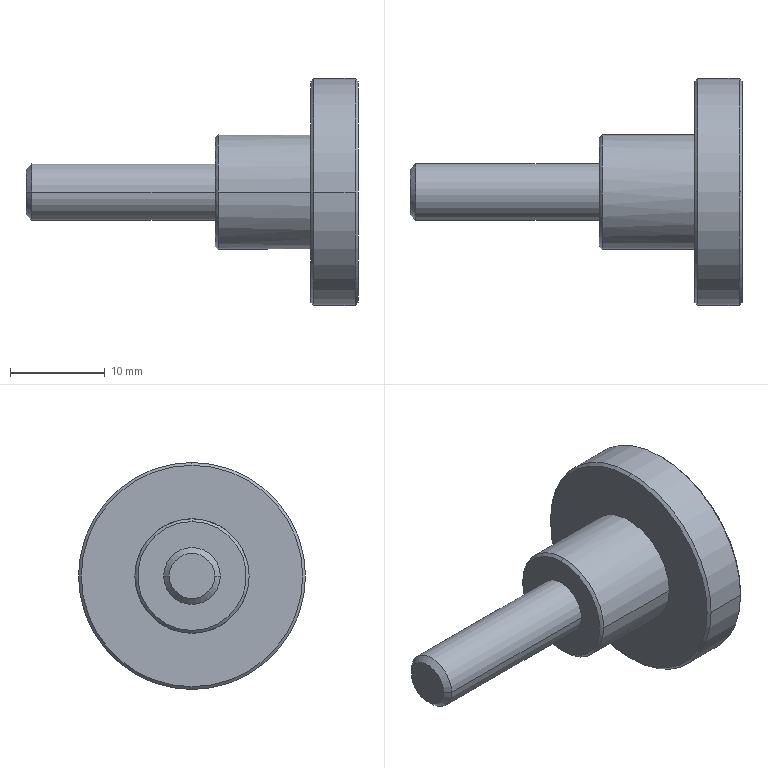Part | SolidWorks | features BaseBody 1 | 1 solid | 18 faces | box 35.1 x 24 x 24 mm | volume 3977 mm3 | cone 8 | cylinder 6 | plane 4 | commonest cylinder face diameters 6 x2 12.1 x2 24 x2
STEP:
#1=CARTESIAN_POINT('',(35.1,0.,-11.7));
#2=VERTEX_POINT('',#1);
#3=CARTESIAN_POINT('',(35.1,0.,11.7));
#4=VERTEX_POINT('',#3);
#5=CARTESIAN_POINT('',(35.1,0.,0.));
#6=DIRECTION('',(1.,0.,0.));
#7=DIRECTION('',(0.,0.,1.));
#8=AXIS2_PLACEMENT_3D('',#5,#6,#7);
#9=CIRCLE('',#8,11.7);
#10=EDGE_CURVE('',#2,#4,#9,.T.);
#11=ORIENTED_EDGE('',*,*,#10,.F.);
#12=CARTESIAN_POINT('',(34.8,0.,-12.));
#13=VERTEX_POINT('',#12);
#14=CARTESIAN_POINT('',(34.8,0.,-12.));
#15=DIRECTION('',(-0.7071,0.,-0.7071));
#16=VECTOR('',#15,1000.);
#17=LINE('',#14,#16);
#18=EDGE_CURVE('',#2,#13,#17,.T.);
#19=ORIENTED_EDGE('',*,*,#18,.T.);
#20=CARTESIAN_POINT('',(34.8,12.,0.));
#21=VERTEX_POINT('',#20);
#22=CARTESIAN_POINT('',(34.8,0.,0.));
#23=DIRECTION('',(1.,0.,0.));
#24=DIRECTION('',(0.,-1.,0.));
#25=AXIS2_PLACEMENT_3D('',#22,#23,#24);
#26=CIRCLE('',#25,12.);
#27=EDGE_CURVE('',#13,#21,#26,.T.);
#28=ORIENTED_EDGE('',*,*,#27,.T.);
#29=CARTESIAN_POINT('',(34.8,0.,12.));
#30=VERTEX_POINT('',#29);
#31=CARTESIAN_POINT('',(34.8,0.,0.));
#32=DIRECTION('',(1.,0.,0.));
#33=DIRECTION('',(0.,-1.,0.));
#34=AXIS2_PLACEMENT_3D('',#31,#32,#33);
#35=CIRCLE('',#34,12.);
#36=EDGE_CURVE('',#21,#30,#35,.T.);
#37=ORIENTED_EDGE('',*,*,#36,.T.);
#38=CARTESIAN_POINT('',(34.8,0.,12.));
#39=DIRECTION('',(-0.7071,0.,0.7071));
#40=VECTOR('',#39,1000.);
#41=LINE('',#38,#40);
#42=EDGE_CURVE('',#4,#30,#41,.T.);
#43=ORIENTED_EDGE('',*,*,#42,.F.);
#44=EDGE_LOOP('',(#11,#19,#28,#37,#43));
#45=FACE_OUTER_BOUND('',#44,.T.);
#46=CARTESIAN_POINT('',(34.8,0.,0.));
#47=DIRECTION('',(-1.,0.,0.));
#48=DIRECTION('',(0.,0.,1.));
#49=AXIS2_PLACEMENT_3D('',#46,#47,#48);
#50=CONICAL_SURFACE('',#49,12.,0.7854);
#51=ADVANCED_FACE('',(#45),#50,.T.);
#52=CARTESIAN_POINT('',(30.4,0.,12.));
#53=VERTEX_POINT('',#52);
#54=CARTESIAN_POINT('',(30.4,-12.,0.));
#55=VERTEX_POINT('',#54);
#56=CARTESIAN_POINT('',(30.4,0.,0.));
#57=DIRECTION('',(1.,0.,0.));
#58=DIRECTION('',(0.,1.,0.));
#59=AXIS2_PLACEMENT_3D('',#56,#57,#58);
#60=CIRCLE('',#59,12.);
#61=EDGE_CURVE('',#53,#55,#60,.T.);
#62=ORIENTED_EDGE('',*,*,#61,.T.);
#63=CARTESIAN_POINT('',(34.8,-12.,0.));
#64=VERTEX_POINT('',#63);
#65=CARTESIAN_POINT('',(35.1,-12.,0.));
#66=DIRECTION('',(1.,0.,0.));
#67=VECTOR('',#66,1000.);
#68=LINE('',#65,#67);
#69=EDGE_CURVE('',#55,#64,#68,.T.);
#70=ORIENTED_EDGE('',*,*,#69,.T.);
#71=CARTESIAN_POINT('',(34.8,0.,0.));
#72=DIRECTION('',(1.,0.,0.));
#73=DIRECTION('',(0.,-1.,0.));
#74=AXIS2_PLACEMENT_3D('',#71,#72,#73);
#75=CIRCLE('',#74,12.);
#76=EDGE_CURVE('',#30,#64,#75,.T.);
#77=ORIENTED_EDGE('',*,*,#76,.F.);
#78=ORIENTED_EDGE('',*,*,#36,.F.);
#79=CARTESIAN_POINT('',(30.4,12.,0.));
#80=VERTEX_POINT('',#79);
#81=CARTESIAN_POINT('',(35.1,12.,0.));
#82=DIRECTION('',(1.,0.,0.));
#83=VECTOR('',#82,1000.);
#84=LINE('',#81,#83);
#85=EDGE_CURVE('',#80,#21,#84,.T.);
#86=ORIENTED_EDGE('',*,*,#85,.F.);
#87=CARTESIAN_POINT('',(30.4,0.,0.));
#88=DIRECTION('',(1.,0.,0.));
#89=DIRECTION('',(0.,1.,0.));
#90=AXIS2_PLACEMENT_3D('',#87,#88,#89);
#91=CIRCLE('',#90,12.);
#92=EDGE_CURVE('',#80,#53,#91,.T.);
#93=ORIENTED_EDGE('',*,*,#92,.T.);
#94=EDGE_LOOP('',(#62,#70,#77,#78,#86,#93));
#95=FACE_OUTER_BOUND('',#94,.T.);
#96=CARTESIAN_POINT('',(35.1,0.,0.));
#97=DIRECTION('',(1.,0.,0.));
#98=DIRECTION('',(0.,1.,0.));
#99=AXIS2_PLACEMENT_3D('',#96,#97,#98);
#100=CYLINDRICAL_SURFACE('',#99,12.);
#101=ADVANCED_FACE('',(#95),#100,.T.);
#102=CARTESIAN_POINT('',(30.1,0.,-11.7));
#103=VERTEX_POINT('',#102);
#104=CARTESIAN_POINT('',(30.1,0.,11.7));
#105=VERTEX_POINT('',#104);
#106=CARTESIAN_POINT('',(30.1,0.,0.));
#107=DIRECTION('',(1.,0.,0.));
#108=DIRECTION('',(0.,0.,-1.));
#109=AXIS2_PLACEMENT_3D('',#106,#107,#108);
#110=CIRCLE('',#109,11.7);
#111=EDGE_CURVE('',#103,#105,#110,.T.);
#112=ORIENTED_EDGE('',*,*,#111,.T.);
#113=CARTESIAN_POINT('',(30.4,0.,12.));
#114=DIRECTION('',(0.7071,0.,0.7071));
#115=VECTOR('',#114,1000.);
#116=LINE('',#113,#115);
#117=EDGE_CURVE('',#105,#53,#116,.T.);
#118=ORIENTED_EDGE('',*,*,#117,.T.);
#119=ORIENTED_EDGE('',*,*,#92,.F.);
#120=CARTESIAN_POINT('',(30.4,0.,-12.));
#121=VERTEX_POINT('',#120);
#122=CARTESIAN_POINT('',(30.4,0.,0.));
#123=DIRECTION('',(1.,0.,0.));
#124=DIRECTION('',(0.,1.,0.));
#125=AXIS2_PLACEMENT_3D('',#122,#123,#124);
#126=CIRCLE('',#125,12.);
#127=EDGE_CURVE('',#121,#80,#126,.T.);
#128=ORIENTED_EDGE('',*,*,#127,.F.);
#129=CARTESIAN_POINT('',(30.4,0.,-12.));
#130=DIRECTION('',(0.7071,0.,-0.7071));
#131=VECTOR('',#130,1000.);
#132=LINE('',#129,#131);
#133=EDGE_CURVE('',#103,#121,#132,.T.);
#134=ORIENTED_EDGE('',*,*,#133,.F.);
#135=EDGE_LOOP('',(#112,#118,#119,#128,#134));
#136=FACE_OUTER_BOUND('',#135,.T.);
#137=CARTESIAN_POINT('',(30.4,0.,0.));
#138=DIRECTION('',(1.,0.,0.));
#139=DIRECTION('',(0.,0.,-1.));
#140=AXIS2_PLACEMENT_3D('',#137,#138,#139);
#141=CONICAL_SURFACE('',#140,12.,0.7854);
#142=ADVANCED_FACE('',(#136),#141,.T.);
#143=CARTESIAN_POINT('',(20.3,0.,6.05));
#144=VERTEX_POINT('',#143);
#145=CARTESIAN_POINT('',(20.3,-6.05,0.));
#146=VERTEX_POINT('',#145);
#147=CARTESIAN_POINT('',(20.3,0.,0.));
#148=DIRECTION('',(1.,0.,0.));
#149=DIRECTION('',(0.,1.,0.));
#150=AXIS2_PLACEMENT_3D('',#147,#148,#149);
#151=CIRCLE('',#150,6.05);
#152=EDGE_CURVE('',#144,#146,#151,.T.);
#153=ORIENTED_EDGE('',*,*,#152,.T.);
#154=CARTESIAN_POINT('',(30.1,-6.05,0.));
#155=VERTEX_POINT('',#154);
#156=CARTESIAN_POINT('',(35.1,-6.05,0.));
#157=DIRECTION('',(1.,0.,0.));
#158=VECTOR('',#157,1000.);
#159=LINE('',#156,#158);
#160=EDGE_CURVE('',#146,#155,#159,.T.);
#161=ORIENTED_EDGE('',*,*,#160,.T.);
#162=CARTESIAN_POINT('',(30.1,6.05,0.));
#163=VERTEX_POINT('',#162);
#164=CARTESIAN_POINT('',(30.1,0.,0.));
#165=DIRECTION('',(1.,0.,0.));
#166=DIRECTION('',(0.,1.,0.));
#167=AXIS2_PLACEMENT_3D('',#164,#165,#166);
#168=CIRCLE('',#167,6.05);
#169=EDGE_CURVE('',#163,#155,#168,.T.);
#170=ORIENTED_EDGE('',*,*,#169,.F.);
#171=CARTESIAN_POINT('',(20.3,6.05,0.));
#172=VERTEX_POINT('',#171);
#173=CARTESIAN_POINT('',(35.1,6.05,0.));
#174=DIRECTION('',(1.,0.,0.));
#175=VECTOR('',#174,1000.);
#176=LINE('',#173,#175);
#177=EDGE_CURVE('',#172,#163,#176,.T.);
#178=ORIENTED_EDGE('',*,*,#177,.F.);
#179=CARTESIAN_POINT('',(20.3,0.,0.));
#180=DIRECTION('',(1.,0.,0.));
#181=DIRECTION('',(0.,1.,0.));
#182=AXIS2_PLACEMENT_3D('',#179,#180,#181);
#183=CIRCLE('',#182,6.05);
#184=EDGE_CURVE('',#172,#144,#183,.T.);
#185=ORIENTED_EDGE('',*,*,#184,.T.);
#186=EDGE_LOOP('',(#153,#161,#170,#178,#185));
#187=FACE_OUTER_BOUND('',#186,.T.);
#188=CARTESIAN_POINT('',(35.1,0.,0.));
#189=DIRECTION('',(1.,0.,0.));
#190=DIRECTION('',(0.,1.,0.));
#191=AXIS2_PLACEMENT_3D('',#188,#189,#190);
#192=CYLINDRICAL_SURFACE('',#191,6.05);
#193=ADVANCED_FACE('',(#187),#192,.T.);
#194=CARTESIAN_POINT('',(20.,0.,-5.75));
#195=VERTEX_POINT('',#194);
#196=CARTESIAN_POINT('',(20.,0.,5.75));
#197=VERTEX_POINT('',#196);
#198=CARTESIAN_POINT('',(20.,0.,0.));
#199=DIRECTION('',(1.,0.,0.));
#200=DIRECTION('',(0.,0.,-1.));
#201=AXIS2_PLACEMENT_3D('',#198,#199,#200);
#202=CIRCLE('',#201,5.75);
#203=EDGE_CURVE('',#195,#197,#202,.T.);
#204=ORIENTED_EDGE('',*,*,#203,.T.);
#205=CARTESIAN_POINT('',(20.3,0.,6.05));
#206=DIRECTION('',(0.7071,0.,0.7071));
#207=VECTOR('',#206,1000.);
#208=LINE('',#205,#207);
#209=EDGE_CURVE('',#197,#144,#208,.T.);
#210=ORIENTED_EDGE('',*,*,#209,.T.);
#211=ORIENTED_EDGE('',*,*,#184,.F.);
#212=CARTESIAN_POINT('',(20.3,0.,-6.05));
#213=VERTEX_POINT('',#212);
#214=CARTESIAN_POINT('',(20.3,0.,0.));
#215=DIRECTION('',(1.,0.,0.));
#216=DIRECTION('',(0.,1.,0.));
#217=AXIS2_PLACEMENT_3D('',#214,#215,#216);
#218=CIRCLE('',#217,6.05);
#219=EDGE_CURVE('',#213,#172,#218,.T.);
#220=ORIENTED_EDGE('',*,*,#219,.F.);
#221=CARTESIAN_POINT('',(20.3,0.,-6.05));
#222=DIRECTION('',(0.7071,0.,-0.7071));
#223=VECTOR('',#222,1000.);
#224=LINE('',#221,#223);
#225=EDGE_CURVE('',#195,#213,#224,.T.);
#226=ORIENTED_EDGE('',*,*,#225,.F.);
#227=EDGE_LOOP('',(#204,#210,#211,#220,#226));
#228=FACE_OUTER_BOUND('',#227,.T.);
#229=CARTESIAN_POINT('',(20.3,0.,0.));
#230=DIRECTION('',(1.,0.,0.));
#231=DIRECTION('',(0.,0.,-1.));
#232=AXIS2_PLACEMENT_3D('',#229,#230,#231);
#233=CONICAL_SURFACE('',#232,6.05,0.7854);
#234=ADVANCED_FACE('',(#228),#233,.T.);
#235=CARTESIAN_POINT('',(0.6,3.,0.));
#236=VERTEX_POINT('',#235);
#237=CARTESIAN_POINT('',(0.6,-3.,0.));
#238=VERTEX_POINT('',#237);
#239=CARTESIAN_POINT('',(0.6,0.,0.));
#240=DIRECTION('',(1.,0.,0.));
#241=DIRECTION('',(0.,1.,0.));
#242=AXIS2_PLACEMENT_3D('',#239,#240,#241);
#243=CIRCLE('',#242,3.);
#244=EDGE_CURVE('',#236,#238,#243,.T.);
#245=ORIENTED_EDGE('',*,*,#244,.T.);
#246=CARTESIAN_POINT('',(20.,-3.,0.));
#247=VERTEX_POINT('',#246);
#248=CARTESIAN_POINT('',(35.1,-3.,0.));
#249=DIRECTION('',(1.,0.,0.));
#250=VECTOR('',#249,1000.);
#251=LINE('',#248,#250);
#252=EDGE_CURVE('',#238,#247,#251,.T.);
#253=ORIENTED_EDGE('',*,*,#252,.T.);
#254=CARTESIAN_POINT('',(20.,3.,0.));
#255=VERTEX_POINT('',#254);
#256=CARTESIAN_POINT('',(20.,0.,0.));
#257=DIRECTION('',(1.,0.,0.));
#258=DIRECTION('',(0.,1.,0.));
#259=AXIS2_PLACEMENT_3D('',#256,#257,#258);
#260=CIRCLE('',#259,3.);
#261=EDGE_CURVE('',#255,#247,#260,.T.);
#262=ORIENTED_EDGE('',*,*,#261,.F.);
#263=CARTESIAN_POINT('',(35.1,3.,0.));
#264=DIRECTION('',(1.,0.,0.));
#265=VECTOR('',#264,1000.);
#266=LINE('',#263,#265);
#267=EDGE_CURVE('',#236,#255,#266,.T.);
#268=ORIENTED_EDGE('',*,*,#267,.F.);
#269=EDGE_LOOP('',(#245,#253,#262,#268));
#270=FACE_OUTER_BOUND('',#269,.T.);
#271=CARTESIAN_POINT('',(35.1,0.,0.));
#272=DIRECTION('',(1.,0.,0.));
#273=DIRECTION('',(0.,1.,0.));
#274=AXIS2_PLACEMENT_3D('',#271,#272,#273);
#275=CYLINDRICAL_SURFACE('',#274,3.);
#276=ADVANCED_FACE('',(#270),#275,.T.);
#277=CARTESIAN_POINT('',(0.,2.4,0.));
#278=VERTEX_POINT('',#277);
#279=CARTESIAN_POINT('',(0.,-2.4,0.));
#280=VERTEX_POINT('',#279);
#281=CARTESIAN_POINT('',(0.,0.,0.));
#282=DIRECTION('',(1.,0.,0.));
#283=DIRECTION('',(0.,1.,0.));
#284=AXIS2_PLACEMENT_3D('',#281,#282,#283);
#285=CIRCLE('',#284,2.4);
#286=EDGE_CURVE('',#278,#280,#285,.T.);
#287=ORIENTED_EDGE('',*,*,#286,.T.);
#288=CARTESIAN_POINT('',(0.6,-3.,0.));
#289=DIRECTION('',(0.7071,-0.7071,0.));
#290=VECTOR('',#289,1000.);
#291=LINE('',#288,#290);
#292=EDGE_CURVE('',#280,#238,#291,.T.);
#293=ORIENTED_EDGE('',*,*,#292,.T.);
#294=ORIENTED_EDGE('',*,*,#244,.F.);
#295=CARTESIAN_POINT('',(0.6,3.,0.));
#296=DIRECTION('',(0.7071,0.7071,0.));
#297=VECTOR('',#296,1000.);
#298=LINE('',#295,#297);
#299=EDGE_CURVE('',#278,#236,#298,.T.);
#300=ORIENTED_EDGE('',*,*,#299,.F.);
#301=EDGE_LOOP('',(#287,#293,#294,#300));
#302=FACE_OUTER_BOUND('',#301,.T.);
#303=CARTESIAN_POINT('',(0.6,0.,0.));
#304=DIRECTION('',(1.,0.,0.));
#305=DIRECTION('',(0.,1.,0.));
#306=AXIS2_PLACEMENT_3D('',#303,#304,#305);
#307=CONICAL_SURFACE('',#306,3.,0.7854);
#308=ADVANCED_FACE('',(#302),#307,.T.);
#309=CARTESIAN_POINT('',(35.1,0.,0.));
#310=DIRECTION('',(1.,0.,0.));
#311=DIRECTION('',(0.,0.,1.));
#312=AXIS2_PLACEMENT_3D('',#309,#310,#311);
#313=CIRCLE('',#312,11.7);
#314=EDGE_CURVE('',#4,#2,#313,.T.);
#315=ORIENTED_EDGE('',*,*,#314,.T.);
#316=ORIENTED_EDGE('',*,*,#10,.T.);
#317=EDGE_LOOP('',(#315,#316));
#318=FACE_OUTER_BOUND('',#317,.T.);
#319=CARTESIAN_POINT('',(35.1,11.7,0.));
#320=DIRECTION('',(1.,0.,0.));
#321=DIRECTION('',(0.,1.,0.));
#322=AXIS2_PLACEMENT_3D('',#319,#320,#321);
#323=PLANE('',#322);
#324=ADVANCED_FACE('',(#318),#323,.T.);
#325=ORIENTED_EDGE('',*,*,#18,.F.);
#326=ORIENTED_EDGE('',*,*,#314,.F.);
#327=ORIENTED_EDGE('',*,*,#42,.T.);
#328=ORIENTED_EDGE('',*,*,#76,.T.);
#329=CARTESIAN_POINT('',(34.8,0.,0.));
#330=DIRECTION('',(1.,0.,0.));
#331=DIRECTION('',(0.,-1.,0.));
#332=AXIS2_PLACEMENT_3D('',#329,#330,#331);
#333=CIRCLE('',#332,12.);
#334=EDGE_CURVE('',#64,#13,#333,.T.);
#335=ORIENTED_EDGE('',*,*,#334,.T.);
#336=EDGE_LOOP('',(#325,#326,#327,#328,#335));
#337=FACE_OUTER_BOUND('',#336,.T.);
#338=CARTESIAN_POINT('',(34.8,0.,0.));
#339=DIRECTION('',(-1.,0.,0.));
#340=DIRECTION('',(0.,0.,1.));
#341=AXIS2_PLACEMENT_3D('',#338,#339,#340);
#342=CONICAL_SURFACE('',#341,12.,0.7854);
#343=ADVANCED_FACE('',(#337),#342,.T.);
#344=ORIENTED_EDGE('',*,*,#69,.F.);
#345=CARTESIAN_POINT('',(30.4,0.,0.));
#346=DIRECTION('',(1.,0.,0.));
#347=DIRECTION('',(0.,1.,0.));
#348=AXIS2_PLACEMENT_3D('',#345,#346,#347);
#349=CIRCLE('',#348,12.);
#350=EDGE_CURVE('',#55,#121,#349,.T.);
#351=ORIENTED_EDGE('',*,*,#350,.T.);
#352=ORIENTED_EDGE('',*,*,#127,.T.);
#353=ORIENTED_EDGE('',*,*,#85,.T.);
#354=ORIENTED_EDGE('',*,*,#27,.F.);
#355=ORIENTED_EDGE('',*,*,#334,.F.);
#356=EDGE_LOOP('',(#344,#351,#352,#353,#354,#355));
#357=FACE_OUTER_BOUND('',#356,.T.);
#358=CARTESIAN_POINT('',(35.1,0.,0.));
#359=DIRECTION('',(1.,0.,0.));
#360=DIRECTION('',(0.,1.,0.));
#361=AXIS2_PLACEMENT_3D('',#358,#359,#360);
#362=CYLINDRICAL_SURFACE('',#361,12.);
#363=ADVANCED_FACE('',(#357),#362,.T.);
#364=ORIENTED_EDGE('',*,*,#117,.F.);
#365=CARTESIAN_POINT('',(30.1,0.,0.));
#366=DIRECTION('',(1.,0.,0.));
#367=DIRECTION('',(0.,0.,-1.));
#368=AXIS2_PLACEMENT_3D('',#365,#366,#367);
#369=CIRCLE('',#368,11.7);
#370=EDGE_CURVE('',#105,#103,#369,.T.);
#371=ORIENTED_EDGE('',*,*,#370,.T.);
#372=ORIENTED_EDGE('',*,*,#133,.T.);
#373=ORIENTED_EDGE('',*,*,#350,.F.);
#374=ORIENTED_EDGE('',*,*,#61,.F.);
#375=EDGE_LOOP('',(#364,#371,#372,#373,#374));
#376=FACE_OUTER_BOUND('',#375,.T.);
#377=CARTESIAN_POINT('',(30.4,0.,0.));
#378=DIRECTION('',(1.,0.,0.));
#379=DIRECTION('',(0.,0.,-1.));
#380=AXIS2_PLACEMENT_3D('',#377,#378,#379);
#381=CONICAL_SURFACE('',#380,12.,0.7854);
#382=ADVANCED_FACE('',(#376),#381,.T.);
#383=ORIENTED_EDGE('',*,*,#111,.F.);
#384=ORIENTED_EDGE('',*,*,#370,.F.);
#385=EDGE_LOOP('',(#383,#384));
#386=FACE_OUTER_BOUND('',#385,.T.);
#387=ORIENTED_EDGE('',*,*,#169,.T.);
#388=CARTESIAN_POINT('',(30.1,0.,0.));
#389=DIRECTION('',(1.,0.,0.));
#390=DIRECTION('',(0.,1.,0.));
#391=AXIS2_PLACEMENT_3D('',#388,#389,#390);
#392=CIRCLE('',#391,6.05);
#393=EDGE_CURVE('',#155,#163,#392,.T.);
#394=ORIENTED_EDGE('',*,*,#393,.T.);
#395=EDGE_LOOP('',(#387,#394));
#396=FACE_BOUND('',#395,.T.);
#397=CARTESIAN_POINT('',(30.1,6.05,0.));
#398=DIRECTION('',(-1.,0.,0.));
#399=DIRECTION('',(0.,-1.,0.));
#400=AXIS2_PLACEMENT_3D('',#397,#398,#399);
#401=PLANE('',#400);
#402=ADVANCED_FACE('',(#386,#396),#401,.T.);
#403=ORIENTED_EDGE('',*,*,#160,.F.);
#404=CARTESIAN_POINT('',(20.3,0.,0.));
#405=DIRECTION('',(1.,0.,0.));
#406=DIRECTION('',(0.,1.,0.));
#407=AXIS2_PLACEMENT_3D('',#404,#405,#406);
#408=CIRCLE('',#407,6.05);
#409=EDGE_CURVE('',#146,#213,#408,.T.);
#410=ORIENTED_EDGE('',*,*,#409,.T.);
#411=ORIENTED_EDGE('',*,*,#219,.T.);
#412=ORIENTED_EDGE('',*,*,#177,.T.);
#413=ORIENTED_EDGE('',*,*,#393,.F.);
#414=EDGE_LOOP('',(#403,#410,#411,#412,#413));
#415=FACE_OUTER_BOUND('',#414,.T.);
#416=CARTESIAN_POINT('',(35.1,0.,0.));
#417=DIRECTION('',(1.,0.,0.));
#418=DIRECTION('',(0.,1.,0.));
#419=AXIS2_PLACEMENT_3D('',#416,#417,#418);
#420=CYLINDRICAL_SURFACE('',#419,6.05);
#421=ADVANCED_FACE('',(#415),#420,.T.);
#422=ORIENTED_EDGE('',*,*,#209,.F.);
#423=CARTESIAN_POINT('',(20.,0.,0.));
#424=DIRECTION('',(1.,0.,0.));
#425=DIRECTION('',(0.,0.,-1.));
#426=AXIS2_PLACEMENT_3D('',#423,#424,#425);
#427=CIRCLE('',#426,5.75);
#428=EDGE_CURVE('',#197,#195,#427,.T.);
#429=ORIENTED_EDGE('',*,*,#428,.T.);
#430=ORIENTED_EDGE('',*,*,#225,.T.);
#431=ORIENTED_EDGE('',*,*,#409,.F.);
#432=ORIENTED_EDGE('',*,*,#152,.F.);
#433=EDGE_LOOP('',(#422,#429,#430,#431,#432));
#434=FACE_OUTER_BOUND('',#433,.T.);
#435=CARTESIAN_POINT('',(20.3,0.,0.));
#436=DIRECTION('',(1.,0.,0.));
#437=DIRECTION('',(0.,0.,-1.));
#438=AXIS2_PLACEMENT_3D('',#435,#436,#437);
#439=CONICAL_SURFACE('',#438,6.05,0.7854);
#440=ADVANCED_FACE('',(#434),#439,.T.);
#441=ORIENTED_EDGE('',*,*,#203,.F.);
#442=ORIENTED_EDGE('',*,*,#428,.F.);
#443=EDGE_LOOP('',(#441,#442));
#444=FACE_OUTER_BOUND('',#443,.T.);
#445=ORIENTED_EDGE('',*,*,#261,.T.);
#446=CARTESIAN_POINT('',(20.,0.,0.));
#447=DIRECTION('',(1.,0.,0.));
#448=DIRECTION('',(0.,1.,0.));
#449=AXIS2_PLACEMENT_3D('',#446,#447,#448);
#450=CIRCLE('',#449,3.);
#451=EDGE_CURVE('',#247,#255,#450,.T.);
#452=ORIENTED_EDGE('',*,*,#451,.T.);
#453=EDGE_LOOP('',(#445,#452));
#454=FACE_BOUND('',#453,.T.);
#455=CARTESIAN_POINT('',(20.,3.,0.));
#456=DIRECTION('',(-1.,0.,0.));
#457=DIRECTION('',(0.,-1.,0.));
#458=AXIS2_PLACEMENT_3D('',#455,#456,#457);
#459=PLANE('',#458);
#460=ADVANCED_FACE('',(#444,#454),#459,.T.);
#461=ORIENTED_EDGE('',*,*,#252,.F.);
#462=CARTESIAN_POINT('',(0.6,0.,0.));
#463=DIRECTION('',(1.,0.,0.));
#464=DIRECTION('',(0.,1.,0.));
#465=AXIS2_PLACEMENT_3D('',#462,#463,#464);
#466=CIRCLE('',#465,3.);
#467=EDGE_CURVE('',#238,#236,#466,.T.);
#468=ORIENTED_EDGE('',*,*,#467,.T.);
#469=ORIENTED_EDGE('',*,*,#267,.T.);
#470=ORIENTED_EDGE('',*,*,#451,.F.);
#471=EDGE_LOOP('',(#461,#468,#469,#470));
#472=FACE_OUTER_BOUND('',#471,.T.);
#473=CARTESIAN_POINT('',(35.1,0.,0.));
#474=DIRECTION('',(1.,0.,0.));
#475=DIRECTION('',(0.,1.,0.));
#476=AXIS2_PLACEMENT_3D('',#473,#474,#475);
#477=CYLINDRICAL_SURFACE('',#476,3.);
#478=ADVANCED_FACE('',(#472),#477,.T.);
#479=ORIENTED_EDGE('',*,*,#292,.F.);
#480=CARTESIAN_POINT('',(0.,0.,0.));
#481=DIRECTION('',(1.,0.,0.));
#482=DIRECTION('',(0.,1.,0.));
#483=AXIS2_PLACEMENT_3D('',#480,#481,#482);
#484=CIRCLE('',#483,2.4);
#485=EDGE_CURVE('',#280,#278,#484,.T.);
#486=ORIENTED_EDGE('',*,*,#485,.T.);
#487=ORIENTED_EDGE('',*,*,#299,.T.);
#488=ORIENTED_EDGE('',*,*,#467,.F.);
#489=EDGE_LOOP('',(#479,#486,#487,#488));
#490=FACE_OUTER_BOUND('',#489,.T.);
#491=CARTESIAN_POINT('',(0.6,0.,0.));
#492=DIRECTION('',(1.,0.,0.));
#493=DIRECTION('',(0.,1.,0.));
#494=AXIS2_PLACEMENT_3D('',#491,#492,#493);
#495=CONICAL_SURFACE('',#494,3.,0.7854);
#496=ADVANCED_FACE('',(#490),#495,.T.);
#497=ORIENTED_EDGE('',*,*,#286,.F.);
#498=ORIENTED_EDGE('',*,*,#485,.F.);
#499=EDGE_LOOP('',(#497,#498));
#500=FACE_OUTER_BOUND('',#499,.T.);
#501=CARTESIAN_POINT('',(0.,0.,0.));
#502=DIRECTION('',(-1.,0.,0.));
#503=DIRECTION('',(0.,-1.,0.));
#504=AXIS2_PLACEMENT_3D('',#501,#502,#503);
#505=PLANE('',#504);
#506=ADVANCED_FACE('',(#500),#505,.T.);
#507=CLOSED_SHELL('',(#51,#101,#142,#193,#234,#276,#308,#324,#343,#363,#382,#402,#421,#440,#460,#478,#496,#506));
#508=MANIFOLD_SOLID_BREP('',#507);
#509=CARTESIAN_POINT('',(0.,0.,0.));
#510=DIRECTION('',(0.,0.,1.));
#511=DIRECTION('',(1.,0.,0.));
#512=AXIS2_PLACEMENT_3D('',#509,#510,#511);
#513=(LENGTH_UNIT()NAMED_UNIT(*)SI_UNIT(.MILLI.,.METRE.));
#514=UNCERTAINTY_MEASURE_WITH_UNIT(LENGTH_MEASURE(0.00001),#513,'','');
#515=(NAMED_UNIT(*)PLANE_ANGLE_UNIT()SI_UNIT($,.RADIAN.));
#516=(NAMED_UNIT(*)SI_UNIT($,.STERADIAN.)SOLID_ANGLE_UNIT());
#517=(GEOMETRIC_REPRESENTATION_CONTEXT(3)GLOBAL_UNCERTAINTY_ASSIGNED_CONTEXT((#514))GLOBAL_UNIT_ASSIGNED_CONTEXT((#513,#515,#516))REPRESENTATION_CONTEXT('',''));
#518=ADVANCED_BREP_SHAPE_REPRESENTATION('',(#508,#512),#517);